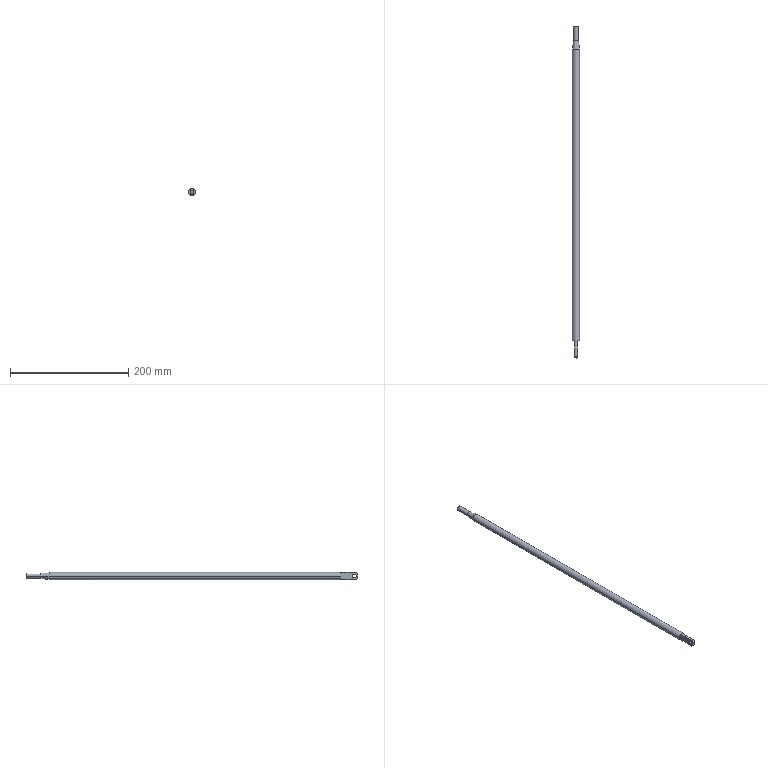Part | SolidWorks | features ICE 3, Chamfer 1, RefAxis 1, Revolution 1 | 1 solid | 16 faces | box 12 x 561 x 12 mm | volume 59373 mm3 | cylinder 6 | plane 6 | cone 4 | commonest cylinder face diameters 6 x2 8 x2 12 x2
STEP:
#1=CARTESIAN_POINT('',(2.,6.,-3.));
#2=VERTEX_POINT('',#1);
#3=CARTESIAN_POINT('',(2.,6.,3.));
#4=VERTEX_POINT('',#3);
#5=CARTESIAN_POINT('',(2.,6.,0.));
#6=DIRECTION('',(-1.,0.,0.));
#7=DIRECTION('',(0.,0.,1.));
#8=AXIS2_PLACEMENT_3D('',#5,#6,#7);
#9=CIRCLE('',#8,3.);
#10=EDGE_CURVE('',#2,#4,#9,.T.);
#11=ORIENTED_EDGE('',*,*,#10,.F.);
#12=CARTESIAN_POINT('',(-2.,6.,-3.));
#13=VERTEX_POINT('',#12);
#14=CARTESIAN_POINT('',(2.,6.,-3.));
#15=DIRECTION('',(-1.,0.,0.));
#16=VECTOR('',#15,1000.);
#17=LINE('',#14,#16);
#18=EDGE_CURVE('',#2,#13,#17,.T.);
#19=ORIENTED_EDGE('',*,*,#18,.T.);
#20=CARTESIAN_POINT('',(-2.,6.,3.));
#21=VERTEX_POINT('',#20);
#22=CARTESIAN_POINT('',(-2.,6.,0.));
#23=DIRECTION('',(-1.,0.,0.));
#24=DIRECTION('',(0.,0.,1.));
#25=AXIS2_PLACEMENT_3D('',#22,#23,#24);
#26=CIRCLE('',#25,3.);
#27=EDGE_CURVE('',#13,#21,#26,.T.);
#28=ORIENTED_EDGE('',*,*,#27,.T.);
#29=CARTESIAN_POINT('',(2.,6.,3.));
#30=DIRECTION('',(-1.,0.,0.));
#31=VECTOR('',#30,1000.);
#32=LINE('',#29,#31);
#33=EDGE_CURVE('',#4,#21,#32,.T.);
#34=ORIENTED_EDGE('',*,*,#33,.F.);
#35=EDGE_LOOP('',(#11,#19,#28,#34));
#36=FACE_OUTER_BOUND('',#35,.T.);
#37=CARTESIAN_POINT('',(2.,6.,0.));
#38=DIRECTION('',(-1.,0.,0.));
#39=DIRECTION('',(0.,0.,1.));
#40=AXIS2_PLACEMENT_3D('',#37,#38,#39);
#41=CYLINDRICAL_SURFACE('',#40,3.);
#42=ADVANCED_FACE('',(#36),#41,.F.);
#43=CARTESIAN_POINT('',(6.,522.,0.));
#44=VERTEX_POINT('',#43);
#45=CARTESIAN_POINT('',(-6.,522.,0.));
#46=VERTEX_POINT('',#45);
#47=CARTESIAN_POINT('',(0.,522.,0.));
#48=DIRECTION('',(0.,-1.,0.));
#49=DIRECTION('',(1.,0.,0.));
#50=AXIS2_PLACEMENT_3D('',#47,#48,#49);
#51=CIRCLE('',#50,6.);
#52=EDGE_CURVE('',#44,#46,#51,.T.);
#53=ORIENTED_EDGE('',*,*,#52,.T.);
#54=CARTESIAN_POINT('',(-6.,29.,0.));
#55=VERTEX_POINT('',#54);
#56=CARTESIAN_POINT('',(-6.,-719.527,0.));
#57=DIRECTION('',(0.,-1.,0.));
#58=VECTOR('',#57,1000.);
#59=LINE('',#56,#58);
#60=EDGE_CURVE('',#46,#55,#59,.T.);
#61=ORIENTED_EDGE('',*,*,#60,.T.);
#62=CARTESIAN_POINT('',(-2.,29.,5.657));
#63=VERTEX_POINT('',#62);
#64=CARTESIAN_POINT('',(0.,29.,0.));
#65=DIRECTION('',(0.,-1.,0.));
#66=DIRECTION('',(0.,0.,1.));
#67=AXIS2_PLACEMENT_3D('',#64,#65,#66);
#68=CIRCLE('',#67,6.);
#69=EDGE_CURVE('',#63,#55,#68,.T.);
#70=ORIENTED_EDGE('',*,*,#69,.F.);
#71=CARTESIAN_POINT('',(-2.,3.,5.657));
#72=VERTEX_POINT('',#71);
#73=CARTESIAN_POINT('',(-2.,-719.527,5.657));
#74=DIRECTION('',(0.,1.,0.));
#75=VECTOR('',#74,1000.);
#76=LINE('',#73,#75);
#77=EDGE_CURVE('',#72,#63,#76,.T.);
#78=ORIENTED_EDGE('',*,*,#77,.F.);
#79=CARTESIAN_POINT('',(2.,3.,5.657));
#80=VERTEX_POINT('',#79);
#81=CARTESIAN_POINT('',(0.,3.,0.));
#82=DIRECTION('',(0.,1.,0.));
#83=DIRECTION('',(1.,0.,0.));
#84=AXIS2_PLACEMENT_3D('',#81,#82,#83);
#85=CIRCLE('',#84,6.);
#86=EDGE_CURVE('',#72,#80,#85,.T.);
#87=ORIENTED_EDGE('',*,*,#86,.T.);
#88=CARTESIAN_POINT('',(2.,29.,5.657));
#89=VERTEX_POINT('',#88);
#90=CARTESIAN_POINT('',(2.,-719.527,5.657));
#91=DIRECTION('',(0.,-1.,0.));
#92=VECTOR('',#91,1000.);
#93=LINE('',#90,#92);
#94=EDGE_CURVE('',#89,#80,#93,.T.);
#95=ORIENTED_EDGE('',*,*,#94,.F.);
#96=CARTESIAN_POINT('',(6.,29.,0.));
#97=VERTEX_POINT('',#96);
#98=CARTESIAN_POINT('',(0.,29.,0.));
#99=DIRECTION('',(0.,-1.,0.));
#100=DIRECTION('',(0.,0.,1.));
#101=AXIS2_PLACEMENT_3D('',#98,#99,#100);
#102=CIRCLE('',#101,6.);
#103=EDGE_CURVE('',#97,#89,#102,.T.);
#104=ORIENTED_EDGE('',*,*,#103,.F.);
#105=CARTESIAN_POINT('',(6.,-719.527,0.));
#106=DIRECTION('',(0.,-1.,0.));
#107=VECTOR('',#106,1000.);
#108=LINE('',#105,#107);
#109=EDGE_CURVE('',#44,#97,#108,.T.);
#110=ORIENTED_EDGE('',*,*,#109,.F.);
#111=EDGE_LOOP('',(#53,#61,#70,#78,#87,#95,#104,#110));
#112=FACE_OUTER_BOUND('',#111,.T.);
#113=CARTESIAN_POINT('',(0.,-719.527,0.));
#114=DIRECTION('',(0.,-1.,0.));
#115=DIRECTION('',(1.,0.,0.));
#116=AXIS2_PLACEMENT_3D('',#113,#114,#115);
#117=CYLINDRICAL_SURFACE('',#116,6.);
#118=ADVANCED_FACE('',(#112),#117,.T.);
#119=CARTESIAN_POINT('',(4.,537.,0.));
#120=VERTEX_POINT('',#119);
#121=CARTESIAN_POINT('',(-4.,537.,0.));
#122=VERTEX_POINT('',#121);
#123=CARTESIAN_POINT('',(0.,537.,0.));
#124=DIRECTION('',(0.,-1.,0.));
#125=DIRECTION('',(1.,0.,0.));
#126=AXIS2_PLACEMENT_3D('',#123,#124,#125);
#127=CIRCLE('',#126,4.);
#128=EDGE_CURVE('',#120,#122,#127,.T.);
#129=ORIENTED_EDGE('',*,*,#128,.T.);
#130=CARTESIAN_POINT('',(-6.,522.,0.));
#131=DIRECTION('',(-0.1322,-0.9912,0.));
#132=VECTOR('',#131,1000.);
#133=LINE('',#130,#132);
#134=EDGE_CURVE('',#122,#46,#133,.T.);
#135=ORIENTED_EDGE('',*,*,#134,.T.);
#136=ORIENTED_EDGE('',*,*,#52,.F.);
#137=CARTESIAN_POINT('',(6.,522.,0.));
#138=DIRECTION('',(0.1322,-0.9912,0.));
#139=VECTOR('',#138,1000.);
#140=LINE('',#137,#139);
#141=EDGE_CURVE('',#120,#44,#140,.T.);
#142=ORIENTED_EDGE('',*,*,#141,.F.);
#143=EDGE_LOOP('',(#129,#135,#136,#142));
#144=FACE_OUTER_BOUND('',#143,.T.);
#145=CARTESIAN_POINT('',(0.,522.,0.));
#146=DIRECTION('',(0.,-1.,0.));
#147=DIRECTION('',(1.,0.,0.));
#148=AXIS2_PLACEMENT_3D('',#145,#146,#147);
#149=CONICAL_SURFACE('',#148,6.,0.1326);
#150=ADVANCED_FACE('',(#144),#149,.T.);
#151=CARTESIAN_POINT('',(4.,561.,0.));
#152=VERTEX_POINT('',#151);
#153=CARTESIAN_POINT('',(-4.,561.,0.));
#154=VERTEX_POINT('',#153);
#155=CARTESIAN_POINT('',(0.,561.,0.));
#156=DIRECTION('',(0.,-1.,0.));
#157=DIRECTION('',(1.,0.,0.));
#158=AXIS2_PLACEMENT_3D('',#155,#156,#157);
#159=CIRCLE('',#158,4.);
#160=EDGE_CURVE('',#152,#154,#159,.T.);
#161=ORIENTED_EDGE('',*,*,#160,.T.);
#162=CARTESIAN_POINT('',(-4.,-719.527,0.));
#163=DIRECTION('',(0.,-1.,0.));
#164=VECTOR('',#163,1000.);
#165=LINE('',#162,#164);
#166=EDGE_CURVE('',#154,#122,#165,.T.);
#167=ORIENTED_EDGE('',*,*,#166,.T.);
#168=ORIENTED_EDGE('',*,*,#128,.F.);
#169=CARTESIAN_POINT('',(4.,-719.527,0.));
#170=DIRECTION('',(0.,-1.,0.));
#171=VECTOR('',#170,1000.);
#172=LINE('',#169,#171);
#173=EDGE_CURVE('',#152,#120,#172,.T.);
#174=ORIENTED_EDGE('',*,*,#173,.F.);
#175=EDGE_LOOP('',(#161,#167,#168,#174));
#176=FACE_OUTER_BOUND('',#175,.T.);
#177=CARTESIAN_POINT('',(0.,-719.527,0.));
#178=DIRECTION('',(0.,-1.,0.));
#179=DIRECTION('',(1.,0.,0.));
#180=AXIS2_PLACEMENT_3D('',#177,#178,#179);
#181=CYLINDRICAL_SURFACE('',#180,4.);
#182=ADVANCED_FACE('',(#176),#181,.T.);
#183=ORIENTED_EDGE('',*,*,#160,.F.);
#184=CARTESIAN_POINT('',(0.,561.,0.));
#185=DIRECTION('',(0.,-1.,0.));
#186=DIRECTION('',(1.,0.,0.));
#187=AXIS2_PLACEMENT_3D('',#184,#185,#186);
#188=CIRCLE('',#187,4.);
#189=EDGE_CURVE('',#154,#152,#188,.T.);
#190=ORIENTED_EDGE('',*,*,#189,.F.);
#191=EDGE_LOOP('',(#183,#190));
#192=FACE_OUTER_BOUND('',#191,.T.);
#193=CARTESIAN_POINT('',(0.,561.,0.));
#194=DIRECTION('',(0.,1.,0.));
#195=DIRECTION('',(-1.,0.,0.));
#196=AXIS2_PLACEMENT_3D('',#193,#194,#195);
#197=PLANE('',#196);
#198=ADVANCED_FACE('',(#192),#197,.T.);
#199=ORIENTED_EDGE('',*,*,#166,.F.);
#200=ORIENTED_EDGE('',*,*,#189,.T.);
#201=ORIENTED_EDGE('',*,*,#173,.T.);
#202=CARTESIAN_POINT('',(0.,537.,0.));
#203=DIRECTION('',(0.,-1.,0.));
#204=DIRECTION('',(1.,0.,0.));
#205=AXIS2_PLACEMENT_3D('',#202,#203,#204);
#206=CIRCLE('',#205,4.);
#207=EDGE_CURVE('',#122,#120,#206,.T.);
#208=ORIENTED_EDGE('',*,*,#207,.F.);
#209=EDGE_LOOP('',(#199,#200,#201,#208));
#210=FACE_OUTER_BOUND('',#209,.T.);
#211=CARTESIAN_POINT('',(0.,-719.527,0.));
#212=DIRECTION('',(0.,-1.,0.));
#213=DIRECTION('',(1.,0.,0.));
#214=AXIS2_PLACEMENT_3D('',#211,#212,#213);
#215=CYLINDRICAL_SURFACE('',#214,4.);
#216=ADVANCED_FACE('',(#210),#215,.T.);
#217=ORIENTED_EDGE('',*,*,#134,.F.);
#218=ORIENTED_EDGE('',*,*,#207,.T.);
#219=ORIENTED_EDGE('',*,*,#141,.T.);
#220=CARTESIAN_POINT('',(0.,522.,0.));
#221=DIRECTION('',(0.,-1.,0.));
#222=DIRECTION('',(1.,0.,0.));
#223=AXIS2_PLACEMENT_3D('',#220,#221,#222);
#224=CIRCLE('',#223,6.);
#225=EDGE_CURVE('',#46,#44,#224,.T.);
#226=ORIENTED_EDGE('',*,*,#225,.F.);
#227=EDGE_LOOP('',(#217,#218,#219,#226));
#228=FACE_OUTER_BOUND('',#227,.T.);
#229=CARTESIAN_POINT('',(0.,522.,0.));
#230=DIRECTION('',(0.,-1.,0.));
#231=DIRECTION('',(1.,0.,0.));
#232=AXIS2_PLACEMENT_3D('',#229,#230,#231);
#233=CONICAL_SURFACE('',#232,6.,0.1326);
#234=ADVANCED_FACE('',(#228),#233,.T.);
#235=ORIENTED_EDGE('',*,*,#60,.F.);
#236=ORIENTED_EDGE('',*,*,#225,.T.);
#237=ORIENTED_EDGE('',*,*,#109,.T.);
#238=CARTESIAN_POINT('',(2.,29.,-5.657));
#239=VERTEX_POINT('',#238);
#240=CARTESIAN_POINT('',(0.,29.,0.));
#241=DIRECTION('',(0.,-1.,0.));
#242=DIRECTION('',(0.,0.,1.));
#243=AXIS2_PLACEMENT_3D('',#240,#241,#242);
#244=CIRCLE('',#243,6.);
#245=EDGE_CURVE('',#239,#97,#244,.T.);
#246=ORIENTED_EDGE('',*,*,#245,.F.);
#247=CARTESIAN_POINT('',(2.,3.,-5.657));
#248=VERTEX_POINT('',#247);
#249=CARTESIAN_POINT('',(2.,-719.527,-5.657));
#250=DIRECTION('',(0.,1.,0.));
#251=VECTOR('',#250,1000.);
#252=LINE('',#249,#251);
#253=EDGE_CURVE('',#248,#239,#252,.T.);
#254=ORIENTED_EDGE('',*,*,#253,.F.);
#255=CARTESIAN_POINT('',(-2.,3.,-5.657));
#256=VERTEX_POINT('',#255);
#257=CARTESIAN_POINT('',(0.,3.,0.));
#258=DIRECTION('',(0.,1.,0.));
#259=DIRECTION('',(1.,0.,0.));
#260=AXIS2_PLACEMENT_3D('',#257,#258,#259);
#261=CIRCLE('',#260,6.);
#262=EDGE_CURVE('',#248,#256,#261,.T.);
#263=ORIENTED_EDGE('',*,*,#262,.T.);
#264=CARTESIAN_POINT('',(-2.,29.,-5.657));
#265=VERTEX_POINT('',#264);
#266=CARTESIAN_POINT('',(-2.,-719.527,-5.657));
#267=DIRECTION('',(0.,-1.,0.));
#268=VECTOR('',#267,1000.);
#269=LINE('',#266,#268);
#270=EDGE_CURVE('',#265,#256,#269,.T.);
#271=ORIENTED_EDGE('',*,*,#270,.F.);
#272=CARTESIAN_POINT('',(0.,29.,0.));
#273=DIRECTION('',(0.,-1.,0.));
#274=DIRECTION('',(0.,0.,1.));
#275=AXIS2_PLACEMENT_3D('',#272,#273,#274);
#276=CIRCLE('',#275,6.);
#277=EDGE_CURVE('',#55,#265,#276,.T.);
#278=ORIENTED_EDGE('',*,*,#277,.F.);
#279=EDGE_LOOP('',(#235,#236,#237,#246,#254,#263,#271,#278));
#280=FACE_OUTER_BOUND('',#279,.T.);
#281=CARTESIAN_POINT('',(0.,-719.527,0.));
#282=DIRECTION('',(0.,-1.,0.));
#283=DIRECTION('',(1.,0.,0.));
#284=AXIS2_PLACEMENT_3D('',#281,#282,#283);
#285=CYLINDRICAL_SURFACE('',#284,6.);
#286=ADVANCED_FACE('',(#280),#285,.T.);
#287=CARTESIAN_POINT('',(2.,0.,2.236));
#288=VERTEX_POINT('',#287);
#289=CARTESIAN_POINT('',(2.,0.,-2.236));
#290=VERTEX_POINT('',#289);
#291=CARTESIAN_POINT('',(2.,0.,0.));
#292=DIRECTION('',(0.,0.,-1.));
#293=VECTOR('',#292,1000.);
#294=LINE('',#291,#293);
#295=EDGE_CURVE('',#288,#290,#294,.T.);
#296=ORIENTED_EDGE('',*,*,#295,.F.);
#297=CARTESIAN_POINT('',(-2.,0.,2.236));
#298=VERTEX_POINT('',#297);
#299=CARTESIAN_POINT('',(0.,0.,0.));
#300=DIRECTION('',(0.,-1.,0.));
#301=DIRECTION('',(1.,0.,0.));
#302=AXIS2_PLACEMENT_3D('',#299,#300,#301);
#303=CIRCLE('',#302,3.);
#304=EDGE_CURVE('',#288,#298,#303,.T.);
#305=ORIENTED_EDGE('',*,*,#304,.T.);
#306=CARTESIAN_POINT('',(-2.,0.,-2.236));
#307=VERTEX_POINT('',#306);
#308=CARTESIAN_POINT('',(-2.,0.,0.));
#309=DIRECTION('',(0.,0.,1.));
#310=VECTOR('',#309,1000.);
#311=LINE('',#308,#310);
#312=EDGE_CURVE('',#307,#298,#311,.T.);
#313=ORIENTED_EDGE('',*,*,#312,.F.);
#314=CARTESIAN_POINT('',(0.,0.,0.));
#315=DIRECTION('',(0.,-1.,0.));
#316=DIRECTION('',(1.,0.,0.));
#317=AXIS2_PLACEMENT_3D('',#314,#315,#316);
#318=CIRCLE('',#317,3.);
#319=EDGE_CURVE('',#307,#290,#318,.T.);
#320=ORIENTED_EDGE('',*,*,#319,.T.);
#321=EDGE_LOOP('',(#296,#305,#313,#320));
#322=FACE_OUTER_BOUND('',#321,.T.);
#323=CARTESIAN_POINT('',(6.,0.,0.));
#324=DIRECTION('',(0.,-1.,0.));
#325=DIRECTION('',(1.,0.,0.));
#326=AXIS2_PLACEMENT_3D('',#323,#324,#325);
#327=PLANE('',#326);
#328=ADVANCED_FACE('',(#322),#327,.T.);
#329=CARTESIAN_POINT('',(-2.,29.,-6.));
#330=DIRECTION('',(0.,0.,1.));
#331=VECTOR('',#330,1000.);
#332=LINE('',#329,#331);
#333=EDGE_CURVE('',#265,#63,#332,.T.);
#334=ORIENTED_EDGE('',*,*,#333,.T.);
#335=ORIENTED_EDGE('',*,*,#69,.T.);
#336=ORIENTED_EDGE('',*,*,#277,.T.);
#337=EDGE_LOOP('',(#334,#335,#336));
#338=FACE_OUTER_BOUND('',#337,.T.);
#339=CARTESIAN_POINT('',(-6.,29.,-6.));
#340=DIRECTION('',(0.,1.,0.));
#341=DIRECTION('',(0.,0.,1.));
#342=AXIS2_PLACEMENT_3D('',#339,#340,#341);
#343=PLANE('',#342);
#344=ADVANCED_FACE('',(#338),#343,.F.);
#345=CARTESIAN_POINT('',(-2.,6.,0.));
#346=DIRECTION('',(-1.,0.,0.));
#347=DIRECTION('',(0.,0.,1.));
#348=AXIS2_PLACEMENT_3D('',#345,#346,#347);
#349=CIRCLE('',#348,3.);
#350=EDGE_CURVE('',#21,#13,#349,.T.);
#351=ORIENTED_EDGE('',*,*,#350,.F.);
#352=ORIENTED_EDGE('',*,*,#27,.F.);
#353=EDGE_LOOP('',(#351,#352));
#354=FACE_BOUND('',#353,.T.);
#355=ORIENTED_EDGE('',*,*,#312,.T.);
#356=CARTESIAN_POINT('',(-2.,0.,2.236));
#357=CARTESIAN_POINT('',(-2.,0.2272,2.541));
#358=CARTESIAN_POINT('',(-2.,0.4662,2.835));
#359=CARTESIAN_POINT('',(-2.,0.9548,3.415));
#360=CARTESIAN_POINT('',(-2.,1.205,3.701));
#361=CARTESIAN_POINT('',(-2.,1.963,4.549));
#362=CARTESIAN_POINT('',(-2.,2.479,5.105));
#363=CARTESIAN_POINT('',(-2.,3.,5.657));
#364=B_SPLINE_CURVE_WITH_KNOTS('',3,(#356,#357,#358,#359,#360,#361,#362,#363),.UNSPECIFIED.,.F.,.F.,(4,2,2,4),(0.,0.001137,0.002275,0.00455),.UNSPECIFIED.);
#365=EDGE_CURVE('',#298,#72,#364,.T.);
#366=ORIENTED_EDGE('',*,*,#365,.T.);
#367=ORIENTED_EDGE('',*,*,#77,.T.);
#368=ORIENTED_EDGE('',*,*,#333,.F.);
#369=ORIENTED_EDGE('',*,*,#270,.T.);
#370=CARTESIAN_POINT('',(-2.,3.,-5.657));
#371=CARTESIAN_POINT('',(-2.,2.479,-5.105));
#372=CARTESIAN_POINT('',(-2.,1.963,-4.549));
#373=CARTESIAN_POINT('',(-2.,1.205,-3.701));
#374=CARTESIAN_POINT('',(-2.,0.9551,-3.416));
#375=CARTESIAN_POINT('',(-2.,0.4665,-2.836));
#376=CARTESIAN_POINT('',(-2.,0.2273,-2.541));
#377=CARTESIAN_POINT('',(-2.,0.,-2.236));
#378=B_SPLINE_CURVE_WITH_KNOTS('',3,(#370,#371,#372,#373,#374,#375,#376,#377),.UNSPECIFIED.,.F.,.F.,(4,2,2,4),(0.,0.002275,0.003412,0.00455),.UNSPECIFIED.);
#379=EDGE_CURVE('',#256,#307,#378,.T.);
#380=ORIENTED_EDGE('',*,*,#379,.T.);
#381=EDGE_LOOP('',(#355,#366,#367,#368,#369,#380));
#382=FACE_OUTER_BOUND('',#381,.T.);
#383=CARTESIAN_POINT('',(-2.,0.,-6.));
#384=DIRECTION('',(1.,0.,0.));
#385=DIRECTION('',(0.,0.,-1.));
#386=AXIS2_PLACEMENT_3D('',#383,#384,#385);
#387=PLANE('',#386);
#388=ADVANCED_FACE('',(#354,#382),#387,.F.);
#389=CARTESIAN_POINT('',(2.,6.,0.));
#390=DIRECTION('',(-1.,0.,0.));
#391=DIRECTION('',(0.,0.,1.));
#392=AXIS2_PLACEMENT_3D('',#389,#390,#391);
#393=CIRCLE('',#392,3.);
#394=EDGE_CURVE('',#4,#2,#393,.T.);
#395=ORIENTED_EDGE('',*,*,#394,.T.);
#396=ORIENTED_EDGE('',*,*,#10,.T.);
#397=EDGE_LOOP('',(#395,#396));
#398=FACE_BOUND('',#397,.T.);
#399=ORIENTED_EDGE('',*,*,#94,.T.);
#400=CARTESIAN_POINT('',(2.,3.,5.657));
#401=CARTESIAN_POINT('',(2.,2.479,5.105));
#402=CARTESIAN_POINT('',(2.,1.963,4.549));
#403=CARTESIAN_POINT('',(2.,1.205,3.701));
#404=CARTESIAN_POINT('',(2.,0.9551,3.416));
#405=CARTESIAN_POINT('',(2.,0.4665,2.836));
#406=CARTESIAN_POINT('',(2.,0.2273,2.541));
#407=CARTESIAN_POINT('',(2.,0.,2.236));
#408=B_SPLINE_CURVE_WITH_KNOTS('',3,(#400,#401,#402,#403,#404,#405,#406,#407),.UNSPECIFIED.,.F.,.F.,(4,2,2,4),(0.,0.002275,0.003412,0.00455),.UNSPECIFIED.);
#409=EDGE_CURVE('',#80,#288,#408,.T.);
#410=ORIENTED_EDGE('',*,*,#409,.T.);
#411=ORIENTED_EDGE('',*,*,#295,.T.);
#412=CARTESIAN_POINT('',(2.,0.,-2.236));
#413=CARTESIAN_POINT('',(2.,0.2272,-2.541));
#414=CARTESIAN_POINT('',(2.,0.4662,-2.835));
#415=CARTESIAN_POINT('',(2.,0.9548,-3.415));
#416=CARTESIAN_POINT('',(2.,1.205,-3.701));
#417=CARTESIAN_POINT('',(2.,1.963,-4.549));
#418=CARTESIAN_POINT('',(2.,2.479,-5.105));
#419=CARTESIAN_POINT('',(2.,3.,-5.657));
#420=B_SPLINE_CURVE_WITH_KNOTS('',3,(#412,#413,#414,#415,#416,#417,#418,#419),.UNSPECIFIED.,.F.,.F.,(4,2,2,4),(0.,0.001137,0.002275,0.00455),.UNSPECIFIED.);
#421=EDGE_CURVE('',#290,#248,#420,.T.);
#422=ORIENTED_EDGE('',*,*,#421,.T.);
#423=ORIENTED_EDGE('',*,*,#253,.T.);
#424=CARTESIAN_POINT('',(2.,29.,-6.));
#425=DIRECTION('',(0.,0.,1.));
#426=VECTOR('',#425,1000.);
#427=LINE('',#424,#426);
#428=EDGE_CURVE('',#239,#89,#427,.T.);
#429=ORIENTED_EDGE('',*,*,#428,.T.);
#430=EDGE_LOOP('',(#399,#410,#411,#422,#423,#429));
#431=FACE_OUTER_BOUND('',#430,.T.);
#432=CARTESIAN_POINT('',(2.,0.,-6.));
#433=DIRECTION('',(-1.,0.,0.));
#434=DIRECTION('',(0.,0.,1.));
#435=AXIS2_PLACEMENT_3D('',#432,#433,#434);
#436=PLANE('',#435);
#437=ADVANCED_FACE('',(#398,#431),#436,.F.);
#438=ORIENTED_EDGE('',*,*,#428,.F.);
#439=ORIENTED_EDGE('',*,*,#245,.T.);
#440=ORIENTED_EDGE('',*,*,#103,.T.);
#441=EDGE_LOOP('',(#438,#439,#440));
#442=FACE_OUTER_BOUND('',#441,.T.);
#443=CARTESIAN_POINT('',(6.,29.,-6.));
#444=DIRECTION('',(0.,1.,0.));
#445=DIRECTION('',(0.,0.,1.));
#446=AXIS2_PLACEMENT_3D('',#443,#444,#445);
#447=PLANE('',#446);
#448=ADVANCED_FACE('',(#442),#447,.F.);
#449=ORIENTED_EDGE('',*,*,#409,.F.);
#450=ORIENTED_EDGE('',*,*,#86,.F.);
#451=ORIENTED_EDGE('',*,*,#365,.F.);
#452=ORIENTED_EDGE('',*,*,#304,.F.);
#453=EDGE_LOOP('',(#449,#450,#451,#452));
#454=FACE_OUTER_BOUND('',#453,.T.);
#455=CARTESIAN_POINT('',(0.,0.,0.));
#456=DIRECTION('',(0.,1.,0.));
#457=DIRECTION('',(-1.,0.,0.));
#458=AXIS2_PLACEMENT_3D('',#455,#456,#457);
#459=CONICAL_SURFACE('',#458,3.,0.7854);
#460=ADVANCED_FACE('',(#454),#459,.T.);
#461=ORIENTED_EDGE('',*,*,#379,.F.);
#462=ORIENTED_EDGE('',*,*,#262,.F.);
#463=ORIENTED_EDGE('',*,*,#421,.F.);
#464=ORIENTED_EDGE('',*,*,#319,.F.);
#465=EDGE_LOOP('',(#461,#462,#463,#464));
#466=FACE_OUTER_BOUND('',#465,.T.);
#467=CARTESIAN_POINT('',(0.,0.,0.));
#468=DIRECTION('',(0.,1.,0.));
#469=DIRECTION('',(-1.,0.,0.));
#470=AXIS2_PLACEMENT_3D('',#467,#468,#469);
#471=CONICAL_SURFACE('',#470,3.,0.7854);
#472=ADVANCED_FACE('',(#466),#471,.T.);
#473=ORIENTED_EDGE('',*,*,#18,.F.);
#474=ORIENTED_EDGE('',*,*,#394,.F.);
#475=ORIENTED_EDGE('',*,*,#33,.T.);
#476=ORIENTED_EDGE('',*,*,#350,.T.);
#477=EDGE_LOOP('',(#473,#474,#475,#476));
#478=FACE_OUTER_BOUND('',#477,.T.);
#479=CARTESIAN_POINT('',(2.,6.,0.));
#480=DIRECTION('',(-1.,0.,0.));
#481=DIRECTION('',(0.,0.,1.));
#482=AXIS2_PLACEMENT_3D('',#479,#480,#481);
#483=CYLINDRICAL_SURFACE('',#482,3.);
#484=ADVANCED_FACE('',(#478),#483,.F.);
#485=CLOSED_SHELL('',(#42,#118,#150,#182,#198,#216,#234,#286,#328,#344,#388,#437,#448,#460,#472,#484));
#486=MANIFOLD_SOLID_BREP('',#485);
#487=CARTESIAN_POINT('',(0.,0.,0.));
#488=DIRECTION('',(0.,0.,1.));
#489=DIRECTION('',(1.,0.,0.));
#490=AXIS2_PLACEMENT_3D('',#487,#488,#489);
#491=(LENGTH_UNIT()NAMED_UNIT(*)SI_UNIT(.MILLI.,.METRE.));
#492=UNCERTAINTY_MEASURE_WITH_UNIT(LENGTH_MEASURE(0.00001),#491,'','');
#493=(NAMED_UNIT(*)PLANE_ANGLE_UNIT()SI_UNIT($,.RADIAN.));
#494=(NAMED_UNIT(*)SI_UNIT($,.STERADIAN.)SOLID_ANGLE_UNIT());
#495=(GEOMETRIC_REPRESENTATION_CONTEXT(3)GLOBAL_UNCERTAINTY_ASSIGNED_CONTEXT((#492))GLOBAL_UNIT_ASSIGNED_CONTEXT((#491,#493,#494))REPRESENTATION_CONTEXT('',''));
#496=ADVANCED_BREP_SHAPE_REPRESENTATION('',(#486,#490),#495);